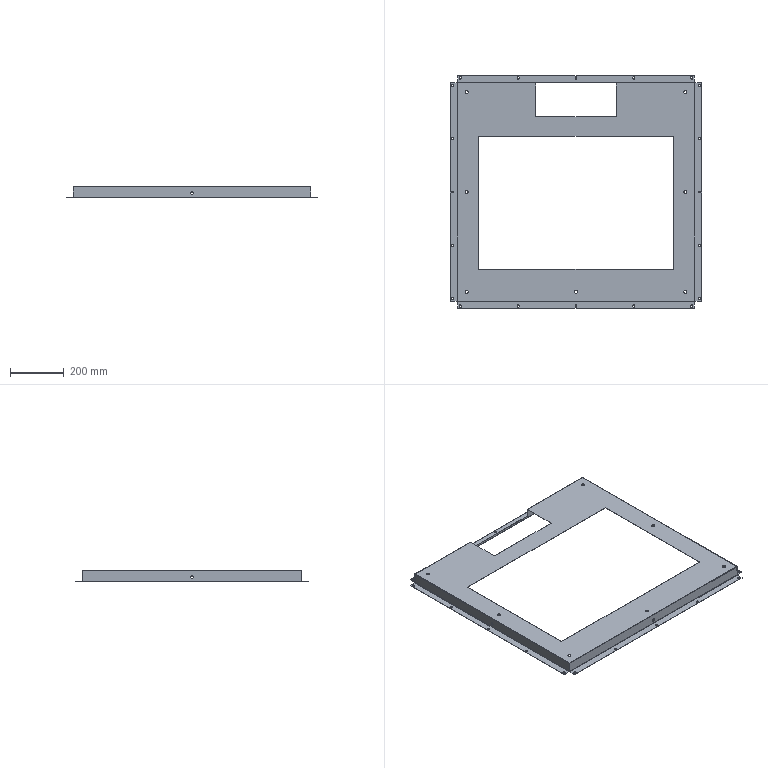Part | 1 solid | 194 faces | box 939 x 869 x 40 mm | volume 532688 mm3 | plane 98 | cylinder 88 | spline 8 | commonest cylinder face diameters 7 x50 11 x14 0.4 x9 2.4 x9 10 x6